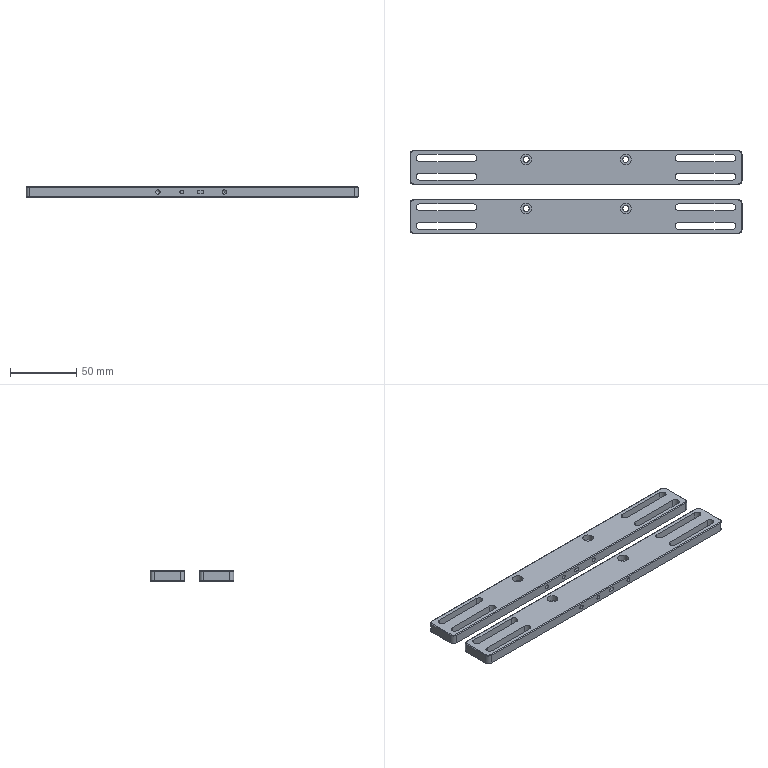NC program | NX | posted with a generic post | part box 250 x 63 x 8 mm
Lines 3836 to 4328 of 4328:
(ZLEVEL_PROFILE_1_COPY_1_COPY_COPY_COPY , TOOL : D6A45)
N7658 T22 M6
N7660 G54
N7662 G17 G0 G90 X7.649 Y-0.541 B0. C0. S7500 M3
N7664 G43 Z30. H22
N7666 Z1.
N7668 G94 G1 Z-1. F1000.
N7670 G3 X8.191 Y0. R0.541
N7672 X7.649 Y-0.541 R-0.541
N7674 X7.909 Y-0.391 R0.3
N7676 G1 Z0.
N7678 G0 Z30.
N7680 X-7.101 Y-0.541
N7682 Z1.
N7684 G1 Z-1.
N7686 X-5.601
N7688 G3 X-5.059 Y0. R0.541
N7690 X-5.601 Y0.541 R0.541
N7692 G1 X-7.101
N7694 G3 X-7.642 Y0. R0.541
N7696 X-7.101 Y-0.541 R0.541
N7698 X-6.581 Y-0.241 R0.6
N7700 G1 Z0.
N7702 G0 Z30.
N7704 X-24.351 Y0.662
N7706 Z1.
N7708 G1 Z-1.
N7710 G3 X-25.013 Y0. R0.662
N7712 X-24.351 Y0.662 R-0.662
N7714 X-24.87 Y0.362 R0.6
N7716 G1 Z0.
N7718 G0 Z30.
N7720 X25.649 Y0.662
N7722 Z1.
N7724 G1 Z-1.
N7726 G3 X24.987 Y0. R0.662
N7728 X25.649 Y0.662 R-0.662
N7730 X25.13 Y0.362 R0.6
N7732 G1 Z0.
N7734 G0 Z30.
N7736 M5
(刀补12 , TOOL : D2)
N7738 T12 M6
N7740 G54
N7742 G17 G0 G90 X-7.175 Y-0.188 B0. C0. S7500 M3
N7744 G43 Z30. H12
N7746 Z-0.429
N7748 G94 G1 Z-1.429 F1000.
N7750 G41 X-7.234 Y-0.269 D12
N7752 X-7.274 Y-0.35
N7754 G3 X-7.101 Y-0.45 R0.2
N7756 G1 X-5.601
N7758 G3 X-5.151 Y0. R0.45
N7760 X-5.601 Y0.45 R0.45
N7762 G1 X-7.101
N7764 G3 X-7.551 Y0. R0.45
N7766 X-7.101 Y-0.45 R0.45
N7768 G1 X-5.71 Z-1.883
N7770 X-5.604 Y-0.444 Z-1.918
N7772 X-5.513 Y-0.434 Z-1.948
N7774 X-5.441 Y-0.411 Z-1.973
N7776 X-5.406 Y-0.399 Z-1.986
N7778 X-5.383 Y-0.384 Z-1.995
N7780 X-5.337 Y-0.354 Z-2.013
N7782 X-5.278 Y-0.302 Z-2.039
N7784 X-5.252 Y-0.273 Z-2.052
N7786 X-5.211 Y-0.208 Z-2.078
N7788 X-5.181 Y-0.135 Z-2.104
N7790 X-5.168 Y-0.098 Z-2.117
N7792 X-5.159 Y-0.021 Z-2.143
N7794 X-5.163 Y0.058 Z-2.169
N7796 X-5.168 Y0.097 Z-2.182
N7798 X-5.193 Y0.169 Z-2.208
N7800 X-5.23 Y0.239 Z-2.234
N7802 X-5.251 Y0.272 Z-2.247
N7804 X-5.305 Y0.327 Z-2.273
N7806 X-5.365 Y0.373 Z-2.298
N7808 X-5.397 Y0.393 Z-2.31
N7810 X-5.422 Y0.404 Z-2.319
N7812 X-5.473 Y0.422 Z-2.338
N7814 X-5.526 Y0.435 Z-2.356
N7816 X-5.591 Y0.443 Z-2.377
N7818 X-5.667 Y0.45 Z-2.403
N7820 X-7.058 Z-2.857
N7822 X-7.101
N7824 G3 X-7.551 Y0. R0.45
N7826 X-7.101 Y-0.45 R0.45
N7828 G1 X-5.71 Z-3.312
N7830 X-5.604 Y-0.444 Z-3.346
N7832 X-5.513 Y-0.434 Z-3.377
N7834 X-5.442 Y-0.411 Z-3.401
N7836 X-5.406 Y-0.399 Z-3.414
N7838 X-5.383 Y-0.384 Z-3.423
N7840 X-5.337 Y-0.354 Z-3.442
N7842 X-5.279 Y-0.302 Z-3.467
N7844 X-5.252 Y-0.273 Z-3.48
N7846 X-5.211 Y-0.208 Z-3.506
N7848 X-5.181 Y-0.135 Z-3.532
N7850 X-5.168 Y-0.099 Z-3.545
N7852 X-5.159 Y-0.021 Z-3.571
N7854 X-5.164 Y0.058 Z-3.598
N7856 X-5.168 Y0.098 Z-3.611
N7858 X-5.193 Y0.169 Z-3.636
N7860 X-5.23 Y0.239 Z-3.662
N7862 X-5.251 Y0.272 Z-3.675
N7864 X-5.268 Y0.291 Z-3.684
N7866 X-5.305 Y0.327 Z-3.701
N7868 X-5.366 Y0.373 Z-3.727
N7870 X-5.398 Y0.394 Z-3.739
N7872 X-5.423 Y0.404 Z-3.748
N7874 X-5.473 Y0.422 Z-3.766
N7876 X-5.526 Y0.435 Z-3.784
N7878 X-5.591 Y0.442 Z-3.806
N7880 X-5.667 Y0.45 Z-3.831
N7882 X-7.058 Z-4.286
N7884 X-7.101
N7886 G3 X-7.551 Y0. R0.45
N7888 X-7.101 Y-0.45 R0.45
N7890 G1 X-5.71 Z-4.74
N7892 X-5.605 Y-0.444 Z-4.775
N7894 X-5.514 Y-0.434 Z-4.805
N7896 X-5.442 Y-0.411 Z-4.83
N7898 X-5.407 Y-0.399 Z-4.842
N7900 X-5.384 Y-0.384 Z-4.852
N7902 X-5.337 Y-0.354 Z-4.87
N7904 X-5.279 Y-0.302 Z-4.896
N7906 X-5.252 Y-0.274 Z-4.909
N7908 X-5.211 Y-0.208 Z-4.935
N7910 X-5.181 Y-0.134 Z-4.961
N7912 X-5.168 Y-0.097 Z-4.974
N7914 X-5.16 Y-0.021 Z-5.
N7916 X-5.164 Y0.058 Z-5.026
N7918 X-5.168 Y0.097 Z-5.039
N7920 X-5.193 Y0.169 Z-5.065
N7922 X-5.23 Y0.238 Z-5.091
N7924 X-5.251 Y0.271 Z-5.104
N7926 X-5.268 Y0.291 Z-5.113
N7928 X-5.305 Y0.327 Z-5.13
N7930 X-5.366 Y0.373 Z-5.155
N7932 X-5.398 Y0.393 Z-5.168
N7934 X-5.422 Y0.405 Z-5.177
N7936 X-5.473 Y0.422 Z-5.195
N7938 X-5.529 Y0.435 Z-5.214
N7940 X-5.594 Y0.443 Z-5.235
N7942 X-5.667 Y0.45 Z-5.26
N7944 X-7.058 Z-5.714
N7946 X-7.101
N7948 G3 X-7.551 Y0. R0.45
N7950 X-7.101 Y-0.45 R0.45
N7952 G1 X-5.71 Z-6.169
N7954 X-5.605 Y-0.444 Z-6.203
N7956 X-5.514 Y-0.434 Z-6.234
N7958 X-5.443 Y-0.411 Z-6.258
N7960 X-5.408 Y-0.399 Z-6.271
N7962 X-5.384 Y-0.384 Z-6.28
N7964 X-5.337 Y-0.354 Z-6.299
N7966 X-5.279 Y-0.302 Z-6.324
N7968 X-5.253 Y-0.274 Z-6.337
N7970 X-5.211 Y-0.208 Z-6.364
N7972 X-5.181 Y-0.135 Z-6.39
N7974 X-5.169 Y-0.098 Z-6.403
N7976 X-5.16 Y-0.021 Z-6.429
N7978 X-5.164 Y0.058 Z-6.455
N7980 X-5.168 Y0.097 Z-6.468
N7982 X-5.193 Y0.169 Z-6.494
N7984 X-5.23 Y0.238 Z-6.519
N7986 X-5.251 Y0.271 Z-6.532
N7988 X-5.268 Y0.29 Z-6.541
N7990 X-5.305 Y0.327 Z-6.558
N7992 X-5.366 Y0.372 Z-6.584
N7994 X-5.397 Y0.393 Z-6.596
N7996 X-5.422 Y0.404 Z-6.605
N7998 X-5.473 Y0.422 Z-6.623
N8000 X-5.529 Y0.435 Z-6.642
N8002 X-5.594 Y0.443 Z-6.664
N8004 X-5.667 Y0.45 Z-6.688
N8006 X-7.058 Z-7.143
N8008 X-7.101
N8010 G3 X-7.551 Y0. R0.45
N8012 X-7.101 Y-0.45 R0.45
N8014 G1 X-5.71 Z-7.597
N8016 X-5.605 Y-0.444 Z-7.632
N8018 X-5.514 Y-0.434 Z-7.662
N8020 X-5.443 Y-0.411 Z-7.687
N8022 X-5.409 Y-0.399 Z-7.699
N8024 X-5.384 Y-0.385 Z-7.708
N8026 X-5.337 Y-0.354 Z-7.727
N8028 X-5.279 Y-0.301 Z-7.753
N8030 X-5.252 Y-0.273 Z-7.766
N8032 X-5.211 Y-0.208 Z-7.792
N8034 X-5.181 Y-0.135 Z-7.818
N8036 X-5.169 Y-0.098 Z-7.831
N8038 X-5.16 Y-0.021 Z-7.857
N8040 X-5.164 Y0.058 Z-7.883
N8042 X-5.169 Y0.096 Z-7.896
N8044 X-5.193 Y0.169 Z-7.922
N8046 X-5.23 Y0.239 Z-7.948
N8048 X-5.251 Y0.272 Z-7.961
N8050 X-5.305 Y0.327 Z-7.987
N8052 X-5.365 Y0.372 Z-8.012
N8054 X-5.397 Y0.392 Z-8.025
N8056 X-5.421 Y0.404 Z-8.034
N8058 X-5.473 Y0.422 Z-8.052
N8060 X-5.528 Y0.435 Z-8.071
N8062 X-5.593 Y0.443 Z-8.092
N8064 X-5.667 Y0.45 Z-8.117
N8066 X-7.058 Z-8.571
N8068 X-7.101
N8070 G3 X-7.551 Y0. R0.45
N8072 X-7.101 Y-0.45 R0.45
N8074 G1 X-5.71 Z-9.026
N8076 X-5.605 Y-0.443 Z-9.06
N8078 X-5.514 Y-0.433 Z-9.091
N8080 X-5.443 Y-0.412 Z-9.115
N8082 X-5.409 Y-0.399 Z-9.127
N8084 X-5.385 Y-0.385 Z-9.137
N8086 X-5.337 Y-0.354 Z-9.156
N8088 X-5.279 Y-0.301 Z-9.182
N8090 X-5.252 Y-0.273 Z-9.195
N8092 X-5.211 Y-0.207 Z-9.221
N8094 X-5.182 Y-0.135 Z-9.247
N8096 X-5.168 Y-0.098 Z-9.26
N8098 X-5.16 Y-0.021 Z-9.286
N8100 X-5.165 Y0.058 Z-9.312
N8102 X-5.168 Y0.098 Z-9.325
N8104 X-5.193 Y0.169 Z-9.351
N8106 X-5.231 Y0.239 Z-9.377
N8108 X-5.251 Y0.272 Z-9.39
N8110 X-5.268 Y0.291 Z-9.398
N8112 X-5.305 Y0.327 Z-9.416
N8114 X-5.366 Y0.373 Z-9.441
N8116 X-5.398 Y0.393 Z-9.454
N8118 X-5.422 Y0.404 Z-9.463
N8120 X-5.473 Y0.422 Z-9.481
N8122 X-5.528 Y0.435 Z-9.499
N8124 X-5.593 Y0.442 Z-9.521
N8126 X-5.667 Y0.45 Z-9.545
N8128 X-7.058 Z-10.
N8130 X-7.101
N8132 G3 X-7.551 Y0. R0.45
N8134 X-7.101 Y-0.45 R0.45
N8136 G1 X-5.601
N8138 G3 X-5.151 Y0. R0.45
N8140 X-5.601 Y0.45 R0.45
N8142 G1 X-7.058
N8144 G3 X-7.231 Y0.35 R0.2
N8146 G1 X-7.307 Y0.218
N8148 G40
N8150 X-7.341 Y0.124
N8152 Z-9.
N8154 G0 Z30.
N8156 X7.575 Y-0.188
N8158 Z-0.429
N8160 G1 Z-1.429
N8162 G41 X7.516 Y-0.269
N8164 X7.476 Y-0.35
N8166 G3 X7.649 Y-0.45 R0.2
N8168 X8.099 Y0. R0.45
N8170 X7.649 Y-0.45 R-0.45
N8172 G1 X7.725 Y-0.435 Z-1.481
N8174 X7.763 Y-0.428 Z-1.507
N8176 X7.833 Y-0.403 Z-1.558
N8178 X7.896 Y-0.365 Z-1.609
N8180 X7.927 Y-0.345 Z-1.634
N8182 X7.946 Y-0.327 Z-1.652
N8184 X7.983 Y-0.289 Z-1.688
N8186 X8.027 Y-0.228 Z-1.74
N8188 X8.047 Y-0.196 Z-1.766
N8190 X8.056 Y-0.172 Z-1.783
N8192 X8.073 Y-0.124 Z-1.818
N8194 X8.088 Y-0.047 Z-1.872
N8196 X8.092 Y-0.009 Z-1.898
N8198 X8.091 Y0.015 Z-1.915
N8200 X8.086 Y0.063 Z-1.948
N8202 X8.067 Y0.141 Z-2.003
N8204 X8.054 Y0.179 Z-2.031
N8206 X8.044 Y0.199 Z-2.046
N8208 X8.02 Y0.238 Z-2.078
N8210 X7.971 Y0.302 Z-2.133
N8212 X7.926 Y0.346 Z-2.176
N8214 X7.888 Y0.371 Z-2.208
N8216 X7.814 Y0.41 Z-2.265
N8218 X7.755 Y0.43 Z-2.308
N8220 X7.712 Y0.437 Z-2.338
N8222 X7.629 Y0.441 Z-2.394
N8224 X7.567 Y0.434 Z-2.438
N8226 X7.525 Y0.423 Z-2.468
N8228 X7.449 Y0.395 Z-2.523
N8230 X7.396 Y0.362 Z-2.566
N8232 X7.36 Y0.334 Z-2.597
N8234 X7.306 Y0.28 Z-2.649
N8236 X7.272 Y0.228 Z-2.692
N8238 X7.247 Y0.184 Z-2.727
N8240 X7.216 Y0.093 Z-2.792
N8242 X7.199 Y0. Z-2.857
N8244 G3 X7.649 Y-0.45 R0.45
N8246 G1 X7.763 Y-0.427 Z-2.936
N8248 X7.786 Y-0.419 Z-2.953
N8250 X7.833 Y-0.403 Z-2.987
N8252 X7.897 Y-0.365 Z-3.037
N8254 X7.927 Y-0.345 Z-3.063
N8256 X7.946 Y-0.327 Z-3.081
N8258 X7.983 Y-0.289 Z-3.117
N8260 X8.027 Y-0.228 Z-3.168
N8262 X8.047 Y-0.196 Z-3.194
N8264 X8.056 Y-0.173 Z-3.211
N8266 X8.072 Y-0.124 Z-3.247
N8268 X8.087 Y-0.046 Z-3.301
N8270 X8.092 Y-0.007 Z-3.328
N8272 X8.091 Y0.016 Z-3.344
N8274 X8.086 Y0.063 Z-3.377
N8276 X8.067 Y0.141 Z-3.431
N8278 X8.054 Y0.179 Z-3.459
N8280 X8.045 Y0.199 Z-3.475
N8282 X8.02 Y0.238 Z-3.506
N8284 X7.969 Y0.304 Z-3.563
N8286 X7.925 Y0.348 Z-3.606
N8288 X7.888 Y0.371 Z-3.636
N8290 X7.811 Y0.41 Z-3.695
N8292 X7.752 Y0.431 Z-3.738
N8294 X7.712 Y0.436 Z-3.766
N8296 X7.626 Y0.441 Z-3.825
N8298 X7.564 Y0.434 Z-3.868
N8300 X7.525 Y0.423 Z-3.896
N8302 X7.447 Y0.393 Z-3.953
N8304 X7.394 Y0.36 Z-3.996
N8306 X7.36 Y0.334 Z-4.026
N8308 X7.306 Y0.281 Z-4.077
N8310 X7.272 Y0.228 Z-4.121
N8312 X7.247 Y0.184 Z-4.156
N8314 X7.217 Y0.093 Z-4.221
N8316 X7.199 Y0. Z-4.286
N8318 G3 X7.649 Y-0.45 R0.45
N8320 G1 X7.763 Y-0.427 Z-4.364
N8322 X7.786 Y-0.419 Z-4.381
N8324 X7.833 Y-0.403 Z-4.416
N8326 X7.896 Y-0.365 Z-4.466
N8328 X7.928 Y-0.345 Z-4.491
N8330 X7.983 Y-0.289 Z-4.545
N8332 X8.027 Y-0.228 Z-4.597
N8334 X8.047 Y-0.196 Z-4.623
N8336 X8.056 Y-0.172 Z-4.64
N8338 X8.072 Y-0.124 Z-4.675
N8340 X8.087 Y-0.047 Z-4.729
N8342 X8.092 Y-0.008 Z-4.756
N8344 X8.091 Y0.016 Z-4.772
N8346 X8.086 Y0.063 Z-4.805
N8348 X8.067 Y0.141 Z-4.86
N8350 X8.054 Y0.178 Z-4.887
N8352 X8.045 Y0.199 Z-4.903
N8354 X8.02 Y0.238 Z-4.935
N8356 X7.969 Y0.304 Z-4.991
N8358 X7.925 Y0.348 Z-5.035
N8360 X7.888 Y0.371 Z-5.065
N8362 X7.811 Y0.41 Z-5.123
N8364 X7.753 Y0.431 Z-5.166
N8366 X7.712 Y0.436 Z-5.195
N8368 X7.627 Y0.441 Z-5.253
N8370 X7.565 Y0.434 Z-5.296
N8372 X7.525 Y0.423 Z-5.325
N8374 X7.447 Y0.394 Z-5.381
N8376 X7.394 Y0.36 Z-5.424
N8378 X7.36 Y0.334 Z-5.455
N8380 X7.306 Y0.281 Z-5.506
N8382 X7.272 Y0.228 Z-5.549
N8384 X7.247 Y0.184 Z-5.584
N8386 X7.217 Y0.093 Z-5.649
N8388 X7.199 Y0. Z-5.714
N8390 G3 X7.649 Y-0.45 R0.45
N8392 G1 X7.762 Y-0.427 Z-5.793
N8394 X7.786 Y-0.419 Z-5.81
N8396 X7.833 Y-0.402 Z-5.844
N8398 X7.897 Y-0.365 Z-5.894
N8400 X7.927 Y-0.345 Z-5.919
N8402 X7.946 Y-0.327 Z-5.938
N8404 X7.983 Y-0.289 Z-5.974
N8406 X8.027 Y-0.227 Z-6.026
N8408 X8.047 Y-0.195 Z-6.052
N8410 X8.056 Y-0.172 Z-6.069
N8412 X8.072 Y-0.124 Z-6.104
N8414 X8.087 Y-0.047 Z-6.158
N8416 X8.091 Y-0.008 Z-6.184
N8418 Y0.015 Z-6.201
N8420 X8.086 Y0.063 Z-6.234
N8422 X8.066 Y0.141 Z-6.289
N8424 X8.053 Y0.179 Z-6.317
N8426 X8.044 Y0.2 Z-6.332
N8428 X8.02 Y0.238 Z-6.364
N8430 X7.969 Y0.303 Z-6.42
N8432 X7.925 Y0.347 Z-6.463
N8434 X7.888 Y0.371 Z-6.494
N8436 X7.812 Y0.41 Z-6.551
N8438 X7.753 Y0.431 Z-6.595
N8440 X7.712 Y0.436 Z-6.623
N8442 X7.627 Y0.441 Z-6.681
N8444 X7.565 Y0.434 Z-6.724
N8446 X7.525 Y0.423 Z-6.753
N8448 X7.447 Y0.394 Z-6.809
N8450 X7.395 Y0.36 Z-6.853
N8452 X7.36 Y0.334 Z-6.883
N8454 X7.307 Y0.281 Z-6.934
N8456 X7.273 Y0.228 Z-6.977
N8458 X7.247 Y0.184 Z-7.013
N8460 X7.217 Y0.093 Z-7.078
N8462 X7.199 Y0. Z-7.143
N8464 G3 X7.649 Y-0.45 R0.45
N8466 G1 X7.762 Y-0.427 Z-7.221
N8468 X7.786 Y-0.419 Z-7.238
N8470 X7.833 Y-0.402 Z-7.273
N8472 X7.896 Y-0.365 Z-7.323
N8474 X7.927 Y-0.345 Z-7.348
N8476 X7.946 Y-0.327 Z-7.366
N8478 X7.983 Y-0.289 Z-7.403
N8480 X8.026 Y-0.227 Z-7.454
N8482 X8.046 Y-0.196 Z-7.48
N8484 X8.056 Y-0.172 Z-7.497
N8486 X8.072 Y-0.124 Z-7.532
N8488 X8.087 Y-0.047 Z-7.586
N8490 X8.092 Y-0.009 Z-7.613
N8492 X8.091 Y0.015 Z-7.629
N8494 X8.085 Y0.063 Z-7.662
N8496 X8.066 Y0.141 Z-7.717
N8498 X8.053 Y0.179 Z-7.745
N8500 X8.044 Y0.199 Z-7.761
N8502 X8.02 Y0.238 Z-7.792
N8504 X7.969 Y0.303 Z-7.848
N8506 X7.925 Y0.347 Z-7.891
N8508 X7.887 Y0.371 Z-7.922
N8510 X7.812 Y0.409 Z-7.98
N8512 X7.753 Y0.43 Z-8.023
N8514 X7.712 Y0.436 Z-8.052
N8516 X7.627 Y0.441 Z-8.109
N8518 X7.566 Y0.434 Z-8.153
N8520 X7.525 Y0.423 Z-8.182
N8522 X7.448 Y0.394 Z-8.238
N8524 X7.395 Y0.36 Z-8.281
N8526 X7.36 Y0.334 Z-8.312
N8528 X7.307 Y0.281 Z-8.362
N8530 X7.273 Y0.229 Z-8.406
N8532 X7.247 Y0.184 Z-8.442
N8534 X7.216 Y0.093 Z-8.506
N8536 X7.199 Y0. Z-8.571
N8538 G3 X7.649 Y-0.45 R0.45
N8540 G1 X7.762 Y-0.427 Z-8.65
N8542 X7.786 Y-0.419 Z-8.667
N8544 X7.833 Y-0.402 Z-8.701
N8546 X7.896 Y-0.365 Z-8.751
N8548 X7.926 Y-0.345 Z-8.776
N8550 X7.945 Y-0.327 Z-8.794
N8552 X7.983 Y-0.289 Z-8.831
N8554 X8.026 Y-0.228 Z-8.882
N8556 X8.046 Y-0.196 Z-8.908
N8558 X8.056 Y-0.172 Z-8.926
N8560 X8.072 Y-0.124 Z-8.961
N8562 X8.087 Y-0.046 Z-9.015
N8564 X8.091 Y-0.007 Z-9.042
N8566 Y0.016 Z-9.058
N8568 X8.085 Y0.063 Z-9.091
N8570 X8.066 Y0.141 Z-9.146
N8572 X8.053 Y0.178 Z-9.173
N8574 X8.044 Y0.199 Z-9.189
N8576 X8.02 Y0.238 Z-9.221
N8578 X7.97 Y0.302 Z-9.276
N8580 X7.925 Y0.346 Z-9.32
N8582 X7.887 Y0.371 Z-9.351
N8584 X7.812 Y0.409 Z-9.408
N8586 X7.754 Y0.43 Z-9.451
N8588 X7.712 Y0.436 Z-9.481
N8590 X7.628 Y0.441 Z-9.538
N8592 X7.566 Y0.434 Z-9.581
N8594 X7.525 Y0.423 Z-9.61
N8596 X7.448 Y0.394 Z-9.666
N8598 X7.396 Y0.36 Z-9.709
N8600 X7.36 Y0.333 Z-9.74
N8602 X7.308 Y0.281 Z-9.791
N8604 X7.273 Y0.229 Z-9.834
N8606 X7.247 Y0.184 Z-9.87
N8608 X7.217 Y0.093 Z-9.935
N8610 X7.199 Y0. Z-10.
N8612 G3 X7.649 Y-0.45 R0.45
N8614 X7.199 Y0. R-0.45
N8616 X7.299 Y-0.173 R0.2
N8618 G1 X7.38 Y-0.133
N8620 G40
N8622 X7.461 Y-0.074
N8624 Z-9.
N8626 G0 Z30.
N8628 M5
N8630 M2